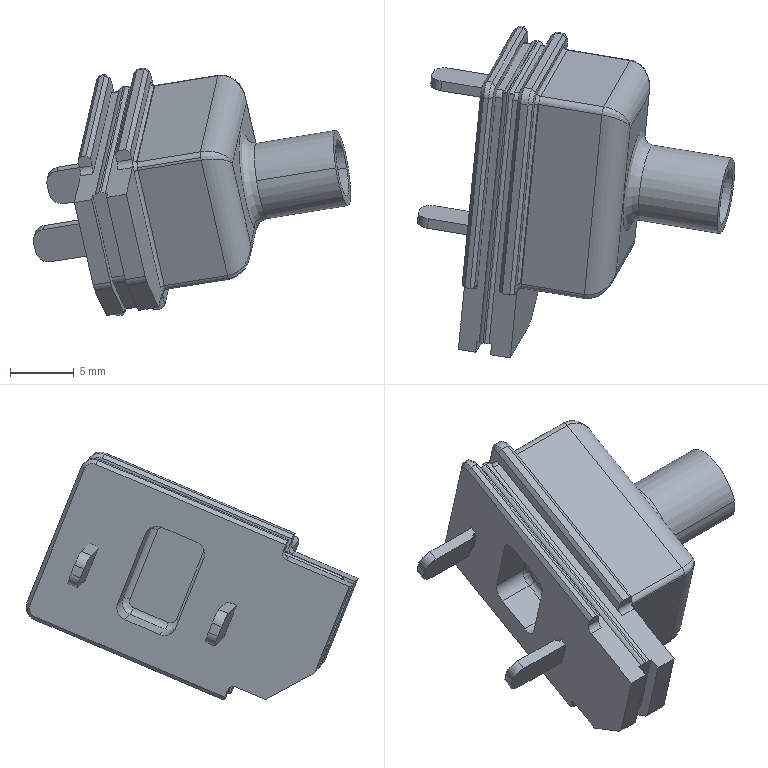Part | STEP file | PN_0016 | 3 solids | 207 faces | box 24.961 x 26.123 x 19.511 mm | volume 2436 mm3 | plane 80 | cylinder 78 | spline 44 | cone 5 | commonest cylinder face diameters 1 x25 2 x17 1.5 x11 0.6 x5 1.009 x5 0.5 x4